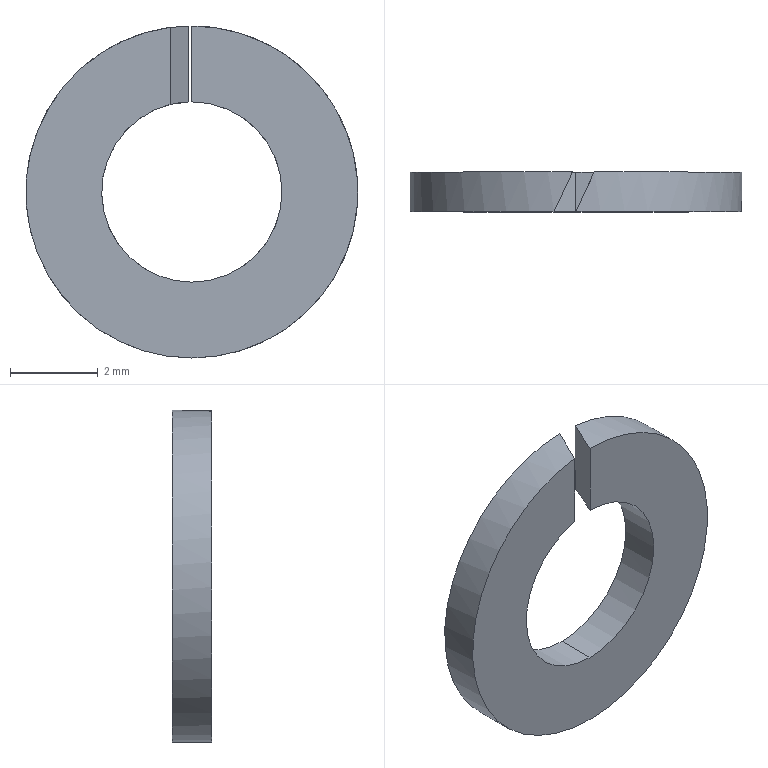Part | SolidWorks | features Extrusion 1, ICE 1, RefAxis 1 | 1 solid | 8 faces | box 7.55 x 0.9 x 7.55 mm | volume 27.638 mm3 | cylinder 4 | plane 4 | commonest cylinder face diameters 4.1 x2 7.55 x2
STEP:
#1=CARTESIAN_POINT('',(0.4197,0.9,2.007));
#2=VERTEX_POINT('',#1);
#3=CARTESIAN_POINT('',(0.,0.9,-2.05));
#4=VERTEX_POINT('',#3);
#5=CARTESIAN_POINT('',(0.,0.9,0.));
#6=DIRECTION('',(0.,1.,0.));
#7=DIRECTION('',(0.,0.,1.));
#8=AXIS2_PLACEMENT_3D('',#5,#6,#7);
#9=CIRCLE('',#8,2.05);
#10=EDGE_CURVE('',#2,#4,#9,.T.);
#11=ORIENTED_EDGE('',*,*,#10,.T.);
#12=CARTESIAN_POINT('',(0.,0.,-2.05));
#13=VERTEX_POINT('',#12);
#14=CARTESIAN_POINT('',(0.,0.9,-2.05));
#15=DIRECTION('',(0.,-1.,0.));
#16=VECTOR('',#15,1000.);
#17=LINE('',#14,#16);
#18=EDGE_CURVE('',#4,#13,#17,.T.);
#19=ORIENTED_EDGE('',*,*,#18,.T.);
#20=CARTESIAN_POINT('',(0.,0.,2.05));
#21=VERTEX_POINT('',#20);
#22=CARTESIAN_POINT('',(0.,0.,0.));
#23=DIRECTION('',(0.,1.,0.));
#24=DIRECTION('',(0.,0.,1.));
#25=AXIS2_PLACEMENT_3D('',#22,#23,#24);
#26=CIRCLE('',#25,2.05);
#27=EDGE_CURVE('',#21,#13,#26,.T.);
#28=ORIENTED_EDGE('',*,*,#27,.F.);
#29=CARTESIAN_POINT('',(0.,0.,2.05));
#30=CARTESIAN_POINT('',(0.1411,0.3027,2.05));
#31=CARTESIAN_POINT('',(0.2815,0.6037,2.035));
#32=CARTESIAN_POINT('',(0.4197,0.9,2.007));
#33=(BOUNDED_CURVE()B_SPLINE_CURVE(3,(#29,#30,#31,#32),.UNSPECIFIED.,.F.,.F.)B_SPLINE_CURVE_WITH_KNOTS((4,4),(1.571,1.777),.UNSPECIFIED.)CURVE()GEOMETRIC_REPRESENTATION_ITEM()RATIONAL_B_SPLINE_CURVE((1.,0.9965,0.9965,1.))REPRESENTATION_ITEM(''));
#34=EDGE_CURVE('',#21,#2,#33,.T.);
#35=ORIENTED_EDGE('',*,*,#34,.T.);
#36=EDGE_LOOP('',(#11,#19,#28,#35));
#37=FACE_OUTER_BOUND('',#36,.T.);
#38=CARTESIAN_POINT('',(0.,0.9,0.));
#39=DIRECTION('',(0.,-1.,0.));
#40=DIRECTION('',(0.,0.,-1.));
#41=AXIS2_PLACEMENT_3D('',#38,#39,#40);
#42=CYLINDRICAL_SURFACE('',#41,2.05);
#43=ADVANCED_FACE('',(#37),#42,.F.);
#44=CARTESIAN_POINT('',(0.,0.9,-3.775));
#45=VERTEX_POINT('',#44);
#46=CARTESIAN_POINT('',(-0.07684,0.9,3.774));
#47=VERTEX_POINT('',#46);
#48=CARTESIAN_POINT('',(0.,0.9,0.));
#49=DIRECTION('',(0.,1.,0.));
#50=DIRECTION('',(0.,0.,1.));
#51=AXIS2_PLACEMENT_3D('',#48,#49,#50);
#52=CIRCLE('',#51,3.775);
#53=EDGE_CURVE('',#45,#47,#52,.T.);
#54=ORIENTED_EDGE('',*,*,#53,.F.);
#55=CARTESIAN_POINT('',(0.,0.,-3.775));
#56=VERTEX_POINT('',#55);
#57=CARTESIAN_POINT('',(0.,0.9,-3.775));
#58=DIRECTION('',(0.,-1.,0.));
#59=VECTOR('',#58,1000.);
#60=LINE('',#57,#59);
#61=EDGE_CURVE('',#45,#56,#60,.T.);
#62=ORIENTED_EDGE('',*,*,#61,.T.);
#63=CARTESIAN_POINT('',(-0.4965,0.,3.742));
#64=VERTEX_POINT('',#63);
#65=CARTESIAN_POINT('',(0.,0.,0.));
#66=DIRECTION('',(0.,1.,0.));
#67=DIRECTION('',(0.,0.,1.));
#68=AXIS2_PLACEMENT_3D('',#65,#66,#67);
#69=CIRCLE('',#68,3.775);
#70=EDGE_CURVE('',#56,#64,#69,.T.);
#71=ORIENTED_EDGE('',*,*,#70,.T.);
#72=CARTESIAN_POINT('',(-0.07684,0.9,3.774));
#73=CARTESIAN_POINT('',(-0.2173,0.5989,3.771));
#74=CARTESIAN_POINT('',(-0.3573,0.2986,3.761));
#75=CARTESIAN_POINT('',(-0.4965,0.,3.742));
#76=(BOUNDED_CURVE()B_SPLINE_CURVE(3,(#72,#73,#74,#75),.UNSPECIFIED.,.F.,.F.)B_SPLINE_CURVE_WITH_KNOTS((4,4),(4.733,4.844),.UNSPECIFIED.)CURVE()GEOMETRIC_REPRESENTATION_ITEM()RATIONAL_B_SPLINE_CURVE((1.,0.999,0.999,1.))REPRESENTATION_ITEM(''));
#77=EDGE_CURVE('',#47,#64,#76,.T.);
#78=ORIENTED_EDGE('',*,*,#77,.F.);
#79=EDGE_LOOP('',(#54,#62,#71,#78));
#80=FACE_OUTER_BOUND('',#79,.T.);
#81=CARTESIAN_POINT('',(0.,0.9,0.));
#82=DIRECTION('',(0.,-1.,0.));
#83=DIRECTION('',(0.,0.,-1.));
#84=AXIS2_PLACEMENT_3D('',#81,#82,#83);
#85=CYLINDRICAL_SURFACE('',#84,3.775);
#86=ADVANCED_FACE('',(#80),#85,.T.);
#87=ORIENTED_EDGE('',*,*,#10,.F.);
#88=CARTESIAN_POINT('',(0.4197,0.9,3.752));
#89=VERTEX_POINT('',#88);
#90=CARTESIAN_POINT('',(0.4197,0.9,3.775));
#91=DIRECTION('',(0.,0.,-1.));
#92=VECTOR('',#91,1000.);
#93=LINE('',#90,#92);
#94=EDGE_CURVE('',#89,#2,#93,.T.);
#95=ORIENTED_EDGE('',*,*,#94,.F.);
#96=CARTESIAN_POINT('',(0.,0.9,0.));
#97=DIRECTION('',(0.,1.,0.));
#98=DIRECTION('',(0.,0.,1.));
#99=AXIS2_PLACEMENT_3D('',#96,#97,#98);
#100=CIRCLE('',#99,3.775);
#101=EDGE_CURVE('',#89,#45,#100,.T.);
#102=ORIENTED_EDGE('',*,*,#101,.T.);
#103=ORIENTED_EDGE('',*,*,#53,.T.);
#104=CARTESIAN_POINT('',(-0.07684,0.9,2.049));
#105=VERTEX_POINT('',#104);
#106=CARTESIAN_POINT('',(-0.07684,0.9,3.775));
#107=DIRECTION('',(0.,0.,-1.));
#108=VECTOR('',#107,1000.);
#109=LINE('',#106,#108);
#110=EDGE_CURVE('',#47,#105,#109,.T.);
#111=ORIENTED_EDGE('',*,*,#110,.T.);
#112=CARTESIAN_POINT('',(0.,0.9,0.));
#113=DIRECTION('',(0.,1.,0.));
#114=DIRECTION('',(0.,0.,1.));
#115=AXIS2_PLACEMENT_3D('',#112,#113,#114);
#116=CIRCLE('',#115,2.05);
#117=EDGE_CURVE('',#4,#105,#116,.T.);
#118=ORIENTED_EDGE('',*,*,#117,.F.);
#119=EDGE_LOOP('',(#87,#95,#102,#103,#111,#118));
#120=FACE_OUTER_BOUND('',#119,.T.);
#121=CARTESIAN_POINT('',(0.,0.9,0.));
#122=DIRECTION('',(0.,1.,0.));
#123=DIRECTION('',(0.,0.,1.));
#124=AXIS2_PLACEMENT_3D('',#121,#122,#123);
#125=PLANE('',#124);
#126=ADVANCED_FACE('',(#120),#125,.T.);
#127=CARTESIAN_POINT('',(0.,0.,3.775));
#128=VERTEX_POINT('',#127);
#129=CARTESIAN_POINT('',(0.,0.,3.775));
#130=DIRECTION('',(0.,0.,-1.));
#131=VECTOR('',#130,1000.);
#132=LINE('',#129,#131);
#133=EDGE_CURVE('',#128,#21,#132,.T.);
#134=ORIENTED_EDGE('',*,*,#133,.T.);
#135=ORIENTED_EDGE('',*,*,#27,.T.);
#136=CARTESIAN_POINT('',(-0.4965,0.,1.989));
#137=VERTEX_POINT('',#136);
#138=CARTESIAN_POINT('',(0.,0.,0.));
#139=DIRECTION('',(0.,1.,0.));
#140=DIRECTION('',(0.,0.,1.));
#141=AXIS2_PLACEMENT_3D('',#138,#139,#140);
#142=CIRCLE('',#141,2.05);
#143=EDGE_CURVE('',#13,#137,#142,.T.);
#144=ORIENTED_EDGE('',*,*,#143,.T.);
#145=CARTESIAN_POINT('',(-0.4965,0.,3.775));
#146=DIRECTION('',(0.,0.,-1.));
#147=VECTOR('',#146,1000.);
#148=LINE('',#145,#147);
#149=EDGE_CURVE('',#64,#137,#148,.T.);
#150=ORIENTED_EDGE('',*,*,#149,.F.);
#151=ORIENTED_EDGE('',*,*,#70,.F.);
#152=CARTESIAN_POINT('',(0.,0.,0.));
#153=DIRECTION('',(0.,1.,0.));
#154=DIRECTION('',(0.,0.,1.));
#155=AXIS2_PLACEMENT_3D('',#152,#153,#154);
#156=CIRCLE('',#155,3.775);
#157=EDGE_CURVE('',#128,#56,#156,.T.);
#158=ORIENTED_EDGE('',*,*,#157,.F.);
#159=EDGE_LOOP('',(#134,#135,#144,#150,#151,#158));
#160=FACE_OUTER_BOUND('',#159,.T.);
#161=CARTESIAN_POINT('',(0.,0.,0.));
#162=DIRECTION('',(0.,1.,0.));
#163=DIRECTION('',(0.,0.,1.));
#164=AXIS2_PLACEMENT_3D('',#161,#162,#163);
#165=PLANE('',#164);
#166=ADVANCED_FACE('',(#160),#165,.F.);
#167=ORIENTED_EDGE('',*,*,#61,.F.);
#168=ORIENTED_EDGE('',*,*,#101,.F.);
#169=CARTESIAN_POINT('',(0.,0.,3.775));
#170=CARTESIAN_POINT('',(0.1403,0.3008,3.775));
#171=CARTESIAN_POINT('',(0.2803,0.6011,3.767));
#172=CARTESIAN_POINT('',(0.4197,0.9,3.752));
#173=(BOUNDED_CURVE()B_SPLINE_CURVE(3,(#169,#170,#171,#172),.UNSPECIFIED.,.F.,.F.)B_SPLINE_CURVE_WITH_KNOTS((4,4),(1.571,1.682),.UNSPECIFIED.)CURVE()GEOMETRIC_REPRESENTATION_ITEM()RATIONAL_B_SPLINE_CURVE((1.,0.999,0.999,1.))REPRESENTATION_ITEM(''));
#174=EDGE_CURVE('',#128,#89,#173,.T.);
#175=ORIENTED_EDGE('',*,*,#174,.F.);
#176=ORIENTED_EDGE('',*,*,#157,.T.);
#177=EDGE_LOOP('',(#167,#168,#175,#176));
#178=FACE_OUTER_BOUND('',#177,.T.);
#179=CARTESIAN_POINT('',(0.,0.9,0.));
#180=DIRECTION('',(0.,-1.,0.));
#181=DIRECTION('',(0.,0.,-1.));
#182=AXIS2_PLACEMENT_3D('',#179,#180,#181);
#183=CYLINDRICAL_SURFACE('',#182,3.775);
#184=ADVANCED_FACE('',(#178),#183,.T.);
#185=ORIENTED_EDGE('',*,*,#18,.F.);
#186=ORIENTED_EDGE('',*,*,#117,.T.);
#187=CARTESIAN_POINT('',(-0.07684,0.9,2.049));
#188=CARTESIAN_POINT('',(-0.2185,0.5961,2.043));
#189=CARTESIAN_POINT('',(-0.3589,0.295,2.023));
#190=CARTESIAN_POINT('',(-0.4965,0.,1.989));
#191=(BOUNDED_CURVE()B_SPLINE_CURVE(3,(#187,#188,#189,#190),.UNSPECIFIED.,.F.,.F.)B_SPLINE_CURVE_WITH_KNOTS((4,4),(4.75,4.957),.UNSPECIFIED.)CURVE()GEOMETRIC_REPRESENTATION_ITEM()RATIONAL_B_SPLINE_CURVE((1.,0.9964,0.9964,1.))REPRESENTATION_ITEM(''));
#192=EDGE_CURVE('',#105,#137,#191,.T.);
#193=ORIENTED_EDGE('',*,*,#192,.T.);
#194=ORIENTED_EDGE('',*,*,#143,.F.);
#195=EDGE_LOOP('',(#185,#186,#193,#194));
#196=FACE_OUTER_BOUND('',#195,.T.);
#197=CARTESIAN_POINT('',(0.,0.9,0.));
#198=DIRECTION('',(0.,-1.,0.));
#199=DIRECTION('',(0.,0.,-1.));
#200=AXIS2_PLACEMENT_3D('',#197,#198,#199);
#201=CYLINDRICAL_SURFACE('',#200,2.05);
#202=ADVANCED_FACE('',(#196),#201,.F.);
#203=ORIENTED_EDGE('',*,*,#77,.T.);
#204=ORIENTED_EDGE('',*,*,#149,.T.);
#205=ORIENTED_EDGE('',*,*,#192,.F.);
#206=ORIENTED_EDGE('',*,*,#110,.F.);
#207=EDGE_LOOP('',(#203,#204,#205,#206));
#208=FACE_OUTER_BOUND('',#207,.T.);
#209=CARTESIAN_POINT('',(-0.07684,0.9,3.775));
#210=DIRECTION('',(0.9063,-0.4226,0.));
#211=DIRECTION('',(0.4226,0.9063,0.));
#212=AXIS2_PLACEMENT_3D('',#209,#210,#211);
#213=PLANE('',#212);
#214=ADVANCED_FACE('',(#208),#213,.T.);
#215=ORIENTED_EDGE('',*,*,#174,.T.);
#216=ORIENTED_EDGE('',*,*,#94,.T.);
#217=ORIENTED_EDGE('',*,*,#34,.F.);
#218=ORIENTED_EDGE('',*,*,#133,.F.);
#219=EDGE_LOOP('',(#215,#216,#217,#218));
#220=FACE_OUTER_BOUND('',#219,.T.);
#221=CARTESIAN_POINT('',(0.,0.,3.775));
#222=DIRECTION('',(-0.9063,0.4226,0.));
#223=DIRECTION('',(-0.4226,-0.9063,0.));
#224=AXIS2_PLACEMENT_3D('',#221,#222,#223);
#225=PLANE('',#224);
#226=ADVANCED_FACE('',(#220),#225,.T.);
#227=CLOSED_SHELL('',(#43,#86,#126,#166,#184,#202,#214,#226));
#228=MANIFOLD_SOLID_BREP('',#227);
#229=CARTESIAN_POINT('',(0.,0.,0.));
#230=DIRECTION('',(0.,0.,1.));
#231=DIRECTION('',(1.,0.,0.));
#232=AXIS2_PLACEMENT_3D('',#229,#230,#231);
#233=(LENGTH_UNIT()NAMED_UNIT(*)SI_UNIT(.MILLI.,.METRE.));
#234=UNCERTAINTY_MEASURE_WITH_UNIT(LENGTH_MEASURE(0.00001),#233,'','');
#235=(NAMED_UNIT(*)PLANE_ANGLE_UNIT()SI_UNIT($,.RADIAN.));
#236=(NAMED_UNIT(*)SI_UNIT($,.STERADIAN.)SOLID_ANGLE_UNIT());
#237=(GEOMETRIC_REPRESENTATION_CONTEXT(3)GLOBAL_UNCERTAINTY_ASSIGNED_CONTEXT((#234))GLOBAL_UNIT_ASSIGNED_CONTEXT((#233,#235,#236))REPRESENTATION_CONTEXT('',''));
#238=ADVANCED_BREP_SHAPE_REPRESENTATION('',(#228,#232),#237);